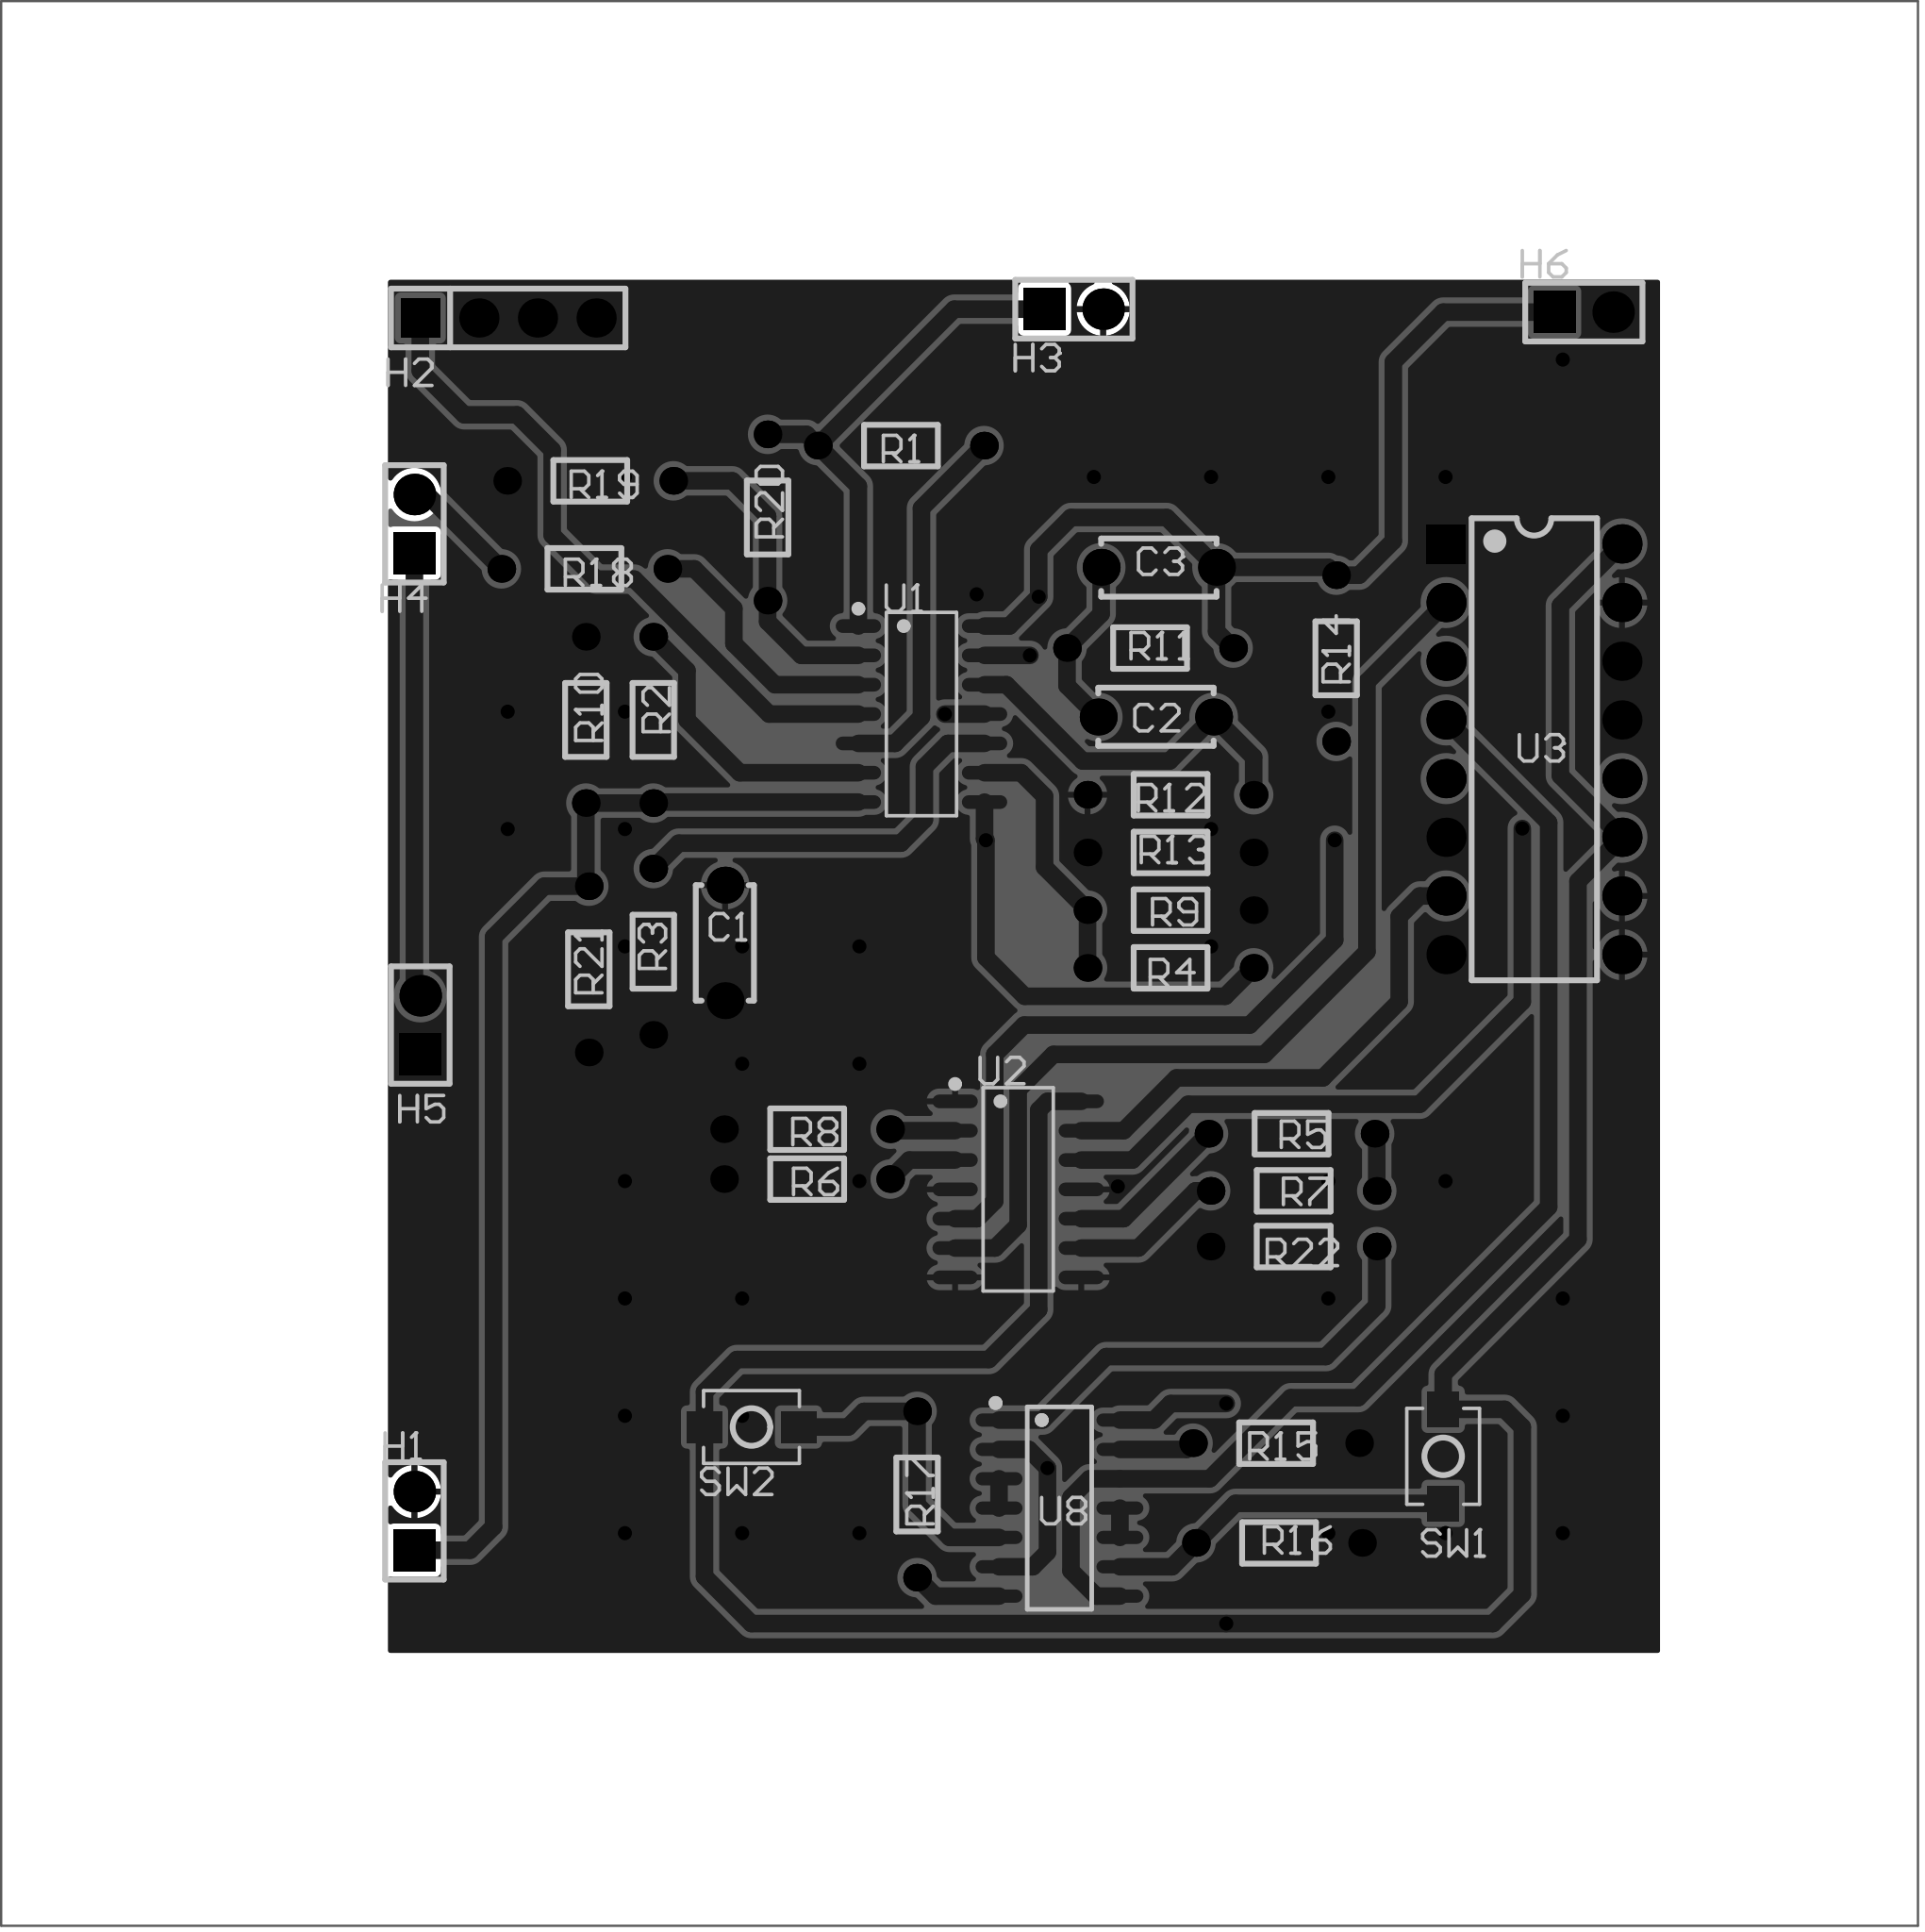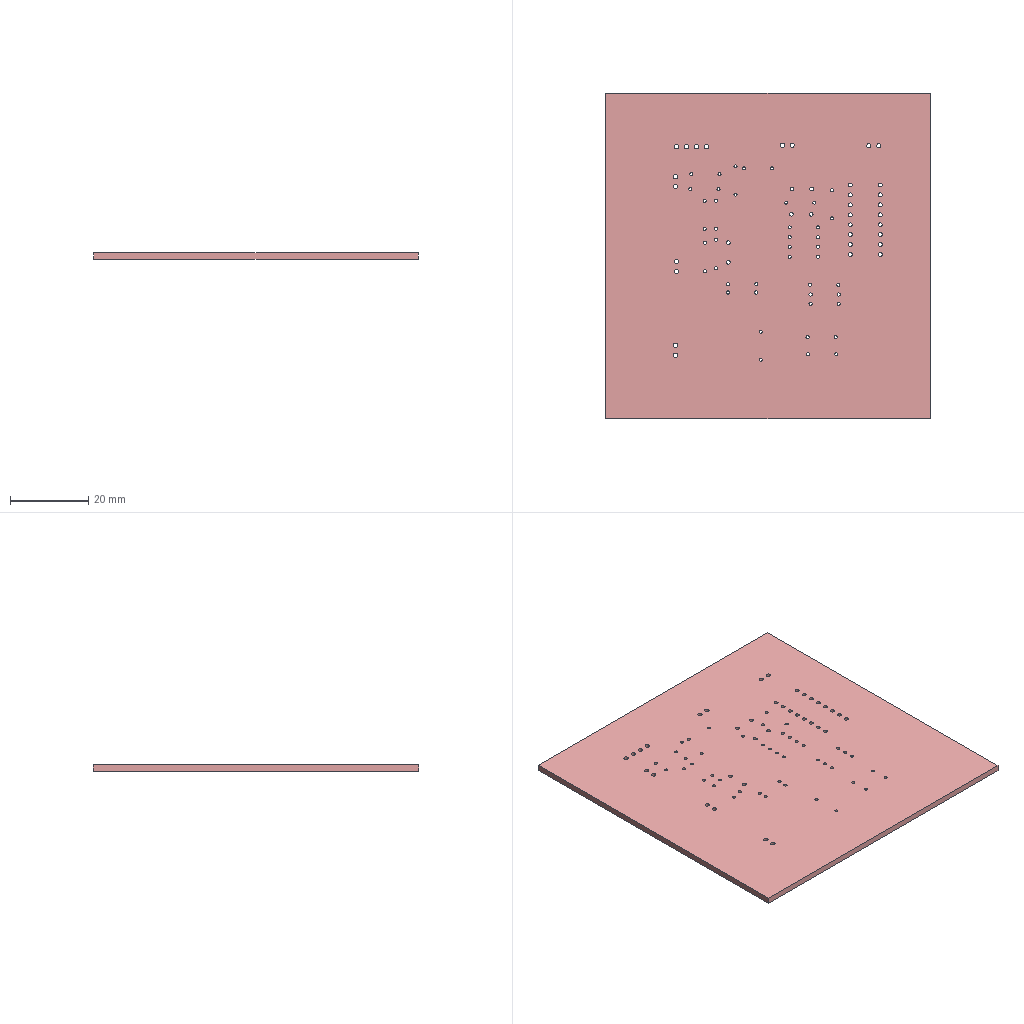Circuit board layout | Altium Designer | box 83.1 x 83.3 x 1.6 mm
Layer stack:
# Altium Designer layer stack of  (unit mm; dielectric type: 0 none, 1 core, 2 prepreg, 3 surface material)
index,name,kind,layer,copper_thickness_mm,dielectric_type,dielectric_thickness_mm,dielectric_material,dielectric_constant
0,Top Paste Mask Layer,other,,,,,,
1,Top Silkscreen Layer,other,,,,,,
2,Top Solder Mask Layer,dielectric,,,3,0.01,,3.3
3,Top Layer,copper,Top Layer,0.035,,,,
4,Dielectric1,dielectric,,,3,1.51,FR4,4.5
5,Bottom Layer,copper,Bottom Layer,0.035,,,,
6,Bottom Solder Mask Layer,dielectric,,,3,0.01,,3.3
7,Bottom Silkscreen Layer,other,,,,,,
8,Bottom Paste Mask Layer,other,,,,,,
# drill layer pairs: low layer,high layer
drill_pair,Top Layer,Bottom Layer
Part placement:
Designator,Comment,Layer,Footprint,Center-X(mm),Center-Y(mm),Rotation
H1,,TopLayer,HDR-TH_2P-P2.54-V-M-1,87.757,87.376,90
H2,,TopLayer,HDR-TH_4P-P2.54-V-M,91.821,139.446,0
H3,,TopLayer,HDR-TH_2P-P2.54-V-M-1,116.332,139.827,0
H4,,TopLayer,HDR-TH_2P-P2.54-V-M-1,87.757,130.534,90
H5,,TopLayer,HDR-TH_2P-P2.54-V-M-1,88.011,108.839,90
H6,,TopLayer,HDR-TH_2P-P2.54-V-M-1,138.43,139.7,0
SW1,,TopLayer,Key_SMD_3x4x2,132.334,90.17,90
SW2,,TopLayer,Key_SMD_3x4x2,102.362,91.44,180
U2,CD4066BD,TopLayer,SOP-14_L8.6-W3.9-P1.27-LS6.0-BL,113.919,101.727,270
U3,NTE74193,TopLayer,PDIP-16_L19.7-W6.6-P2.54-LS7.6-BL,136.271,120.777,270
U1,LM324ADR,TopLayer,SOP-14_L8.6-W3.9-P1.27-LS6.0-BL,109.728,122.301,270
U8,SN74LS00DR,TopLayer,SOIC-14_L8.7-W3.9-P1.27-LS6.0-BL,115.708,87.93,270
C1,10nF,TopLayer,CAP-TH_L5.0-W2.5-P5.00-D1.0,101.219,112.395,270
C2,100nF,TopLayer,CAP-TH_L5.0-W2.5-P5.00-D1.0,119.888,122.174,180
C3,100nF,TopLayer,CAP-TH_L5.0-W2.5-P5.00-D1.0,120.015,128.651,0
R1,15K,TopLayer,Res_1/8W,108.839,133.921,0
R2,1200K,TopLayer,Res_1/8W,98.107,122.047,270
R3,47K,TopLayer,Res_1/8W,98.108,112.014,90
R4,120K,TopLayer,Res_1/8W,120.523,111.315,0
R5,80K,TopLayer,Res_1/8W,125.765,104.135,0
R6,40K,TopLayer,Res_1/8W,104.775,102.172,180
R7,20K,TopLayer,Res_1/8W,125.857,101.663,0
R8,10K,TopLayer,Res_1/8W,104.775,104.331,180
R9,230K,TopLayer,Res_1/8W,120.523,113.813,180
R10,80K,TopLayer,Res_1/8W,95.186,122.047,270
R11,15K,TopLayer,Res_1/8W,119.634,125.158,0
R12,15K,TopLayer,Res_1/8W,120.523,118.808,0
R13,80K,TopLayer,Res_1/8W,120.523,116.31,180
R14,51K,TopLayer,Res_1/8W,127.698,124.714,270
R15,15K,TopLayer,Res_1/8W,125.095,90.741,0
R16,15K,TopLayer,Res_1/8W,125.222,86.424,180
R17,1K,TopLayer,Res_1/8W,109.538,88.519,90
R18,10K,TopLayer,Res_1/8W,95.123,128.587,0
R19,10K,TopLayer,Res_1/8W,95.377,132.397,0
R20,90K,TopLayer,Res_1/8W,103.061,130.81,90
R21,120K,TopLayer,Res_1/8W,95.313,111.252,270
R22,15K,TopLayer,Res_1/8W,125.857,99.251,180
Pad and via stacks:
# Altium Designer via and pad stacks of  (unit mm). Each distinct definition once, with the count of objects using it.
# via: kind,start_layer,end_layer,hole_mm,diameter_mm,mode(0 simple;1 top-mid-bottom;2 full stack),diameter_per_layer,count,example_net
# pad: kind,layer,hole_mm,hole_type(0 round;1 square;2 slot),plating,top_size,top_shape(1 round;2 rect;3 octagon;9 rounded rect),mid_size,bottom_size,mode,footprint,size_per_layer,count,example
pad,Multi-Layer,1.1,0,plated,1.8x1.8,1,1.8x1.8,1.8x1.8,0,HDR-TH_2P-P2.54-V-M-1,,5,H1.2
pad,Multi-Layer,1.1,0,plated,1.8x1.8,2,1.8x1.8,1.8x1.8,0,HDR-TH_2P-P2.54-V-M-1,,5,H1.1
pad,Multi-Layer,1.1,0,plated,1.7x1.7,2,1.7x1.7,1.7x1.7,0,HDR-TH_4P-P2.54-V-M,,1,H2.1
pad,Multi-Layer,1.1,0,plated,1.7x1.7,1,1.7x1.7,1.7x1.7,0,HDR-TH_4P-P2.54-V-M,,3,H2.2
pad,Multi-Layer,1,0,plated,1.7x1.7,2,1.7x1.7,1.7x1.7,0,PDIP-16_L19.7-W6.6-P2.54-LS7.6-BL,,1,U3.1
pad,Multi-Layer,1,0,plated,1.7x1.7,1,1.7x1.7,1.7x1.7,0,PDIP-16_L19.7-W6.6-P2.54-LS7.6-BL,,15,U3.2
pad,Multi-Layer,1,0,plated,1.6x1.6,1,1.6x1.6,1.6x1.6,0,CAP-TH_L5.0-W2.5-P5.00-D1.0,,6,C1.1
pad,Multi-Layer,0.8001,0,plated,1.199x1.199,1,1.199x1.199,1.199x1.199,0,Res_1/8W,,44,R1.1
pad,Top Layer,0,0,plated,1.53x1.36,2,1.53x1.36,1.53x1.36,0,Key_SMD_3x4x2,,4,SW1.1
pad,Top Layer,0,0,plated,0.595x1.968,1,0.595x1.968,0.595x1.968,0,SOP-14_L8.6-W3.9-P1.27-LS6.0-BL,,28,U2.1
pad,Top Layer,0,0,plated,0.574x2.038,1,0.574x2.038,0.574x2.038,0,SOIC-14_L8.7-W3.9-P1.27-LS6.0-BL,,14,U8.8
via,Top Layer,Bottom Layer,0.3048,0.61,0,,46,5V
Copper pours:
name,layer,net,type(0 solid;1 hatched;2 none)
Top Layer-GND,Top Layer,GND,0
Bottom Layer-GND,Bottom Layer,GND,0